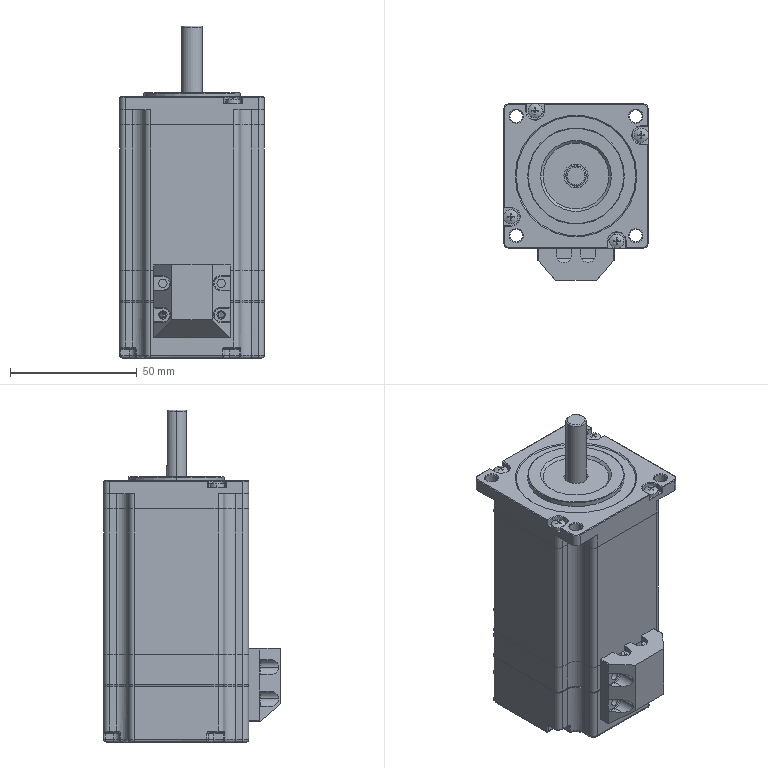Part | SolidWorks | 10 solids | 1966 faces | box 57.15 x 69.65 x 131 mm | volume 178571 mm3 | cone 1297 | cylinder 294 | plane 288 | spline 87 | commonest cylinder face diameters 1 x57 4.6 x40 0.6 x31 3.2 x27 9.5 x20 2 x16